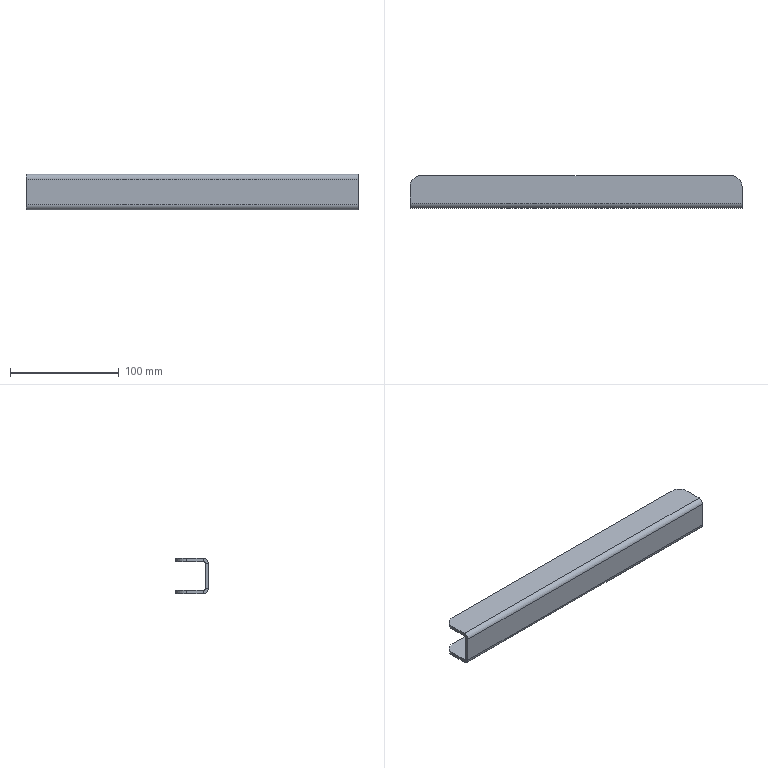Part | NX | features BREP 1 | 1 solid | 26 faces | box 304.8 x 29.997 x 32.461 mm | volume 76853 mm3 | plane 18 | cylinder 8 | commonest cylinder face diameters 19.964 x4 3.175 x2 9.22 x2
STEP:
#1=CARTESIAN_POINT('',(-152.4,0.,11.62));
#2=VERTEX_POINT('',#1);
#3=CARTESIAN_POINT('',(152.4,0.,11.62));
#4=VERTEX_POINT('',#3);
#5=CARTESIAN_POINT('',(-152.4,0.,11.62));
#6=DIRECTION('',(1.,0.,0.));
#7=VECTOR('',#6,1000.);
#8=LINE('',#5,#7);
#9=EDGE_CURVE('',#2,#4,#8,.T.);
#10=ORIENTED_EDGE('',*,*,#9,.T.);
#11=CARTESIAN_POINT('',(152.4,0.,-11.62));
#12=VERTEX_POINT('',#11);
#13=CARTESIAN_POINT('',(152.4,0.,11.62));
#14=DIRECTION('',(0.,0.,-1.));
#15=VECTOR('',#14,1000.);
#16=LINE('',#13,#15);
#17=EDGE_CURVE('',#4,#12,#16,.T.);
#18=ORIENTED_EDGE('',*,*,#17,.T.);
#19=CARTESIAN_POINT('',(-152.4,0.,-11.62));
#20=VERTEX_POINT('',#19);
#21=CARTESIAN_POINT('',(152.4,0.,-11.62));
#22=DIRECTION('',(-1.,0.,0.));
#23=VECTOR('',#22,1000.);
#24=LINE('',#21,#23);
#25=EDGE_CURVE('',#12,#20,#24,.T.);
#26=ORIENTED_EDGE('',*,*,#25,.T.);
#27=CARTESIAN_POINT('',(-152.4,0.,-11.62));
#28=DIRECTION('',(0.,0.,1.));
#29=VECTOR('',#28,1000.);
#30=LINE('',#27,#29);
#31=EDGE_CURVE('',#20,#2,#30,.T.);
#32=ORIENTED_EDGE('',*,*,#31,.T.);
#33=EDGE_LOOP('',(#10,#18,#26,#32));
#34=FACE_BOUND('',#33,.T.);
#35=CARTESIAN_POINT('',(0.,0.,0.));
#36=DIRECTION('',(0.,1.,0.));
#37=DIRECTION('',(1.,0.,0.));
#38=AXIS2_PLACEMENT_3D('',#35,#36,#37);
#39=PLANE('',#38);
#40=ADVANCED_FACE('',(#34),#39,.T.);
#41=CARTESIAN_POINT('',(-152.4,-3.023,-11.62));
#42=VERTEX_POINT('',#41);
#43=CARTESIAN_POINT('',(-152.4,0.,-11.62));
#44=DIRECTION('',(0.,-1.,0.));
#45=VECTOR('',#44,1000.);
#46=LINE('',#43,#45);
#47=EDGE_CURVE('',#20,#42,#46,.T.);
#48=ORIENTED_EDGE('',*,*,#47,.T.);
#49=CARTESIAN_POINT('',(-152.4,-3.023,11.62));
#50=VERTEX_POINT('',#49);
#51=CARTESIAN_POINT('',(-152.4,-3.023,-11.62));
#52=DIRECTION('',(0.,0.,1.));
#53=VECTOR('',#52,1000.);
#54=LINE('',#51,#53);
#55=EDGE_CURVE('',#42,#50,#54,.T.);
#56=ORIENTED_EDGE('',*,*,#55,.T.);
#57=CARTESIAN_POINT('',(-152.4,0.,11.62));
#58=DIRECTION('',(0.,-1.,0.));
#59=VECTOR('',#58,1000.);
#60=LINE('',#57,#59);
#61=EDGE_CURVE('',#2,#50,#60,.T.);
#62=ORIENTED_EDGE('',*,*,#61,.F.);
#63=ORIENTED_EDGE('',*,*,#31,.F.);
#64=EDGE_LOOP('',(#48,#56,#62,#63));
#65=FACE_BOUND('',#64,.T.);
#66=CARTESIAN_POINT('',(-152.4,-1.511,0.));
#67=DIRECTION('',(-1.,0.,0.));
#68=DIRECTION('',(0.,0.,1.));
#69=AXIS2_PLACEMENT_3D('',#66,#67,#68);
#70=PLANE('',#69);
#71=ADVANCED_FACE('',(#65),#70,.T.);
#72=ORIENTED_EDGE('',*,*,#61,.T.);
#73=CARTESIAN_POINT('',(-152.4,1.587,16.231));
#74=VERTEX_POINT('',#73);
#75=CARTESIAN_POINT('',(-152.4,1.587,11.62));
#76=DIRECTION('',(1.,0.,0.));
#77=DIRECTION('',(0.,0.,1.));
#78=AXIS2_PLACEMENT_3D('',#75,#76,#77);
#79=CIRCLE('',#78,4.61);
#80=EDGE_CURVE('',#74,#50,#79,.T.);
#81=ORIENTED_EDGE('',*,*,#80,.F.);
#82=CARTESIAN_POINT('',(-152.4,1.587,13.208));
#83=VERTEX_POINT('',#82);
#84=CARTESIAN_POINT('',(-152.4,1.587,13.208));
#85=DIRECTION('',(0.,0.,1.));
#86=VECTOR('',#85,1000.);
#87=LINE('',#84,#86);
#88=EDGE_CURVE('',#83,#74,#87,.T.);
#89=ORIENTED_EDGE('',*,*,#88,.F.);
#90=CARTESIAN_POINT('',(-152.4,1.587,11.62));
#91=DIRECTION('',(1.,0.,0.));
#92=DIRECTION('',(0.,0.,1.));
#93=AXIS2_PLACEMENT_3D('',#90,#91,#92);
#94=CIRCLE('',#93,1.587);
#95=EDGE_CURVE('',#83,#2,#94,.T.);
#96=ORIENTED_EDGE('',*,*,#95,.T.);
#97=EDGE_LOOP('',(#72,#81,#89,#96));
#98=FACE_BOUND('',#97,.T.);
#99=CARTESIAN_POINT('',(-152.4,-0.6037,13.812));
#100=DIRECTION('',(1.,0.,0.));
#101=DIRECTION('',(0.,1.,0.));
#102=AXIS2_PLACEMENT_3D('',#99,#100,#101);
#103=PLANE('',#102);
#104=ADVANCED_FACE('',(#98),#103,.F.);
#105=CARTESIAN_POINT('',(152.4,1.587,13.208));
#106=VERTEX_POINT('',#105);
#107=CARTESIAN_POINT('',(152.4,1.587,11.62));
#108=DIRECTION('',(1.,0.,0.));
#109=DIRECTION('',(0.,0.,1.));
#110=AXIS2_PLACEMENT_3D('',#107,#108,#109);
#111=CIRCLE('',#110,1.587);
#112=EDGE_CURVE('',#106,#4,#111,.T.);
#113=ORIENTED_EDGE('',*,*,#112,.T.);
#114=ORIENTED_EDGE('',*,*,#9,.F.);
#115=ORIENTED_EDGE('',*,*,#95,.F.);
#116=CARTESIAN_POINT('',(-152.4,1.587,13.208));
#117=DIRECTION('',(1.,0.,0.));
#118=VECTOR('',#117,1000.);
#119=LINE('',#116,#118);
#120=EDGE_CURVE('',#83,#106,#119,.T.);
#121=ORIENTED_EDGE('',*,*,#120,.T.);
#122=EDGE_LOOP('',(#113,#114,#115,#121));
#123=FACE_BOUND('',#122,.T.);
#124=CARTESIAN_POINT('',(-152.4,1.587,11.62));
#125=DIRECTION('',(1.,0.,0.));
#126=DIRECTION('',(0.,0.,1.));
#127=AXIS2_PLACEMENT_3D('',#124,#125,#126);
#128=CYLINDRICAL_SURFACE('',#127,1.587);
#129=ADVANCED_FACE('',(#123),#128,.F.);
#130=CARTESIAN_POINT('',(152.4,16.942,13.208));
#131=VERTEX_POINT('',#130);
#132=CARTESIAN_POINT('',(152.4,1.587,13.208));
#133=DIRECTION('',(0.,1.,0.));
#134=VECTOR('',#133,1000.);
#135=LINE('',#132,#134);
#136=EDGE_CURVE('',#106,#131,#135,.T.);
#137=ORIENTED_EDGE('',*,*,#136,.F.);
#138=ORIENTED_EDGE('',*,*,#120,.F.);
#139=CARTESIAN_POINT('',(-152.4,16.942,13.208));
#140=VERTEX_POINT('',#139);
#141=CARTESIAN_POINT('',(-152.4,16.942,13.208));
#142=DIRECTION('',(0.,-1.,0.));
#143=VECTOR('',#142,1000.);
#144=LINE('',#141,#143);
#145=EDGE_CURVE('',#140,#83,#144,.T.);
#146=ORIENTED_EDGE('',*,*,#145,.F.);
#147=CARTESIAN_POINT('',(-142.418,26.924,13.208));
#148=VERTEX_POINT('',#147);
#149=CARTESIAN_POINT('',(-142.418,16.942,13.208));
#150=DIRECTION('',(0.,0.,-1.));
#151=DIRECTION('',(-1.,0.,0.));
#152=AXIS2_PLACEMENT_3D('',#149,#150,#151);
#153=CIRCLE('',#152,9.982);
#154=EDGE_CURVE('',#140,#148,#153,.T.);
#155=ORIENTED_EDGE('',*,*,#154,.T.);
#156=CARTESIAN_POINT('',(142.418,26.924,13.208));
#157=VERTEX_POINT('',#156);
#158=CARTESIAN_POINT('',(142.418,26.924,13.208));
#159=DIRECTION('',(-1.,0.,0.));
#160=VECTOR('',#159,1000.);
#161=LINE('',#158,#160);
#162=EDGE_CURVE('',#157,#148,#161,.T.);
#163=ORIENTED_EDGE('',*,*,#162,.F.);
#164=CARTESIAN_POINT('',(142.418,16.942,13.208));
#165=DIRECTION('',(0.,0.,-1.));
#166=DIRECTION('',(0.,1.,0.));
#167=AXIS2_PLACEMENT_3D('',#164,#165,#166);
#168=CIRCLE('',#167,9.982);
#169=EDGE_CURVE('',#157,#131,#168,.T.);
#170=ORIENTED_EDGE('',*,*,#169,.T.);
#171=EDGE_LOOP('',(#137,#138,#146,#155,#163,#170));
#172=FACE_BOUND('',#171,.T.);
#173=CARTESIAN_POINT('',(-79.98,0.,13.208));
#174=DIRECTION('',(0.,0.,1.));
#175=DIRECTION('',(1.,0.,0.));
#176=AXIS2_PLACEMENT_3D('',#173,#174,#175);
#177=PLANE('',#176);
#178=ADVANCED_FACE('',(#172),#177,.F.);
#179=CARTESIAN_POINT('',(152.4,16.942,16.231));
#180=VERTEX_POINT('',#179);
#181=CARTESIAN_POINT('',(142.418,26.924,16.231));
#182=VERTEX_POINT('',#181);
#183=CARTESIAN_POINT('',(142.418,16.942,16.231));
#184=DIRECTION('',(0.,0.,1.));
#185=DIRECTION('',(1.,0.,0.));
#186=AXIS2_PLACEMENT_3D('',#183,#184,#185);
#187=CIRCLE('',#186,9.982);
#188=EDGE_CURVE('',#180,#182,#187,.T.);
#189=ORIENTED_EDGE('',*,*,#188,.F.);
#190=CARTESIAN_POINT('',(152.4,16.942,16.231));
#191=DIRECTION('',(0.,0.,-1.));
#192=VECTOR('',#191,1000.);
#193=LINE('',#190,#192);
#194=EDGE_CURVE('',#180,#131,#193,.T.);
#195=ORIENTED_EDGE('',*,*,#194,.T.);
#196=ORIENTED_EDGE('',*,*,#169,.F.);
#197=CARTESIAN_POINT('',(142.418,26.924,16.231));
#198=DIRECTION('',(0.,0.,-1.));
#199=VECTOR('',#198,1000.);
#200=LINE('',#197,#199);
#201=EDGE_CURVE('',#182,#157,#200,.T.);
#202=ORIENTED_EDGE('',*,*,#201,.F.);
#203=EDGE_LOOP('',(#189,#195,#196,#202));
#204=FACE_BOUND('',#203,.T.);
#205=CARTESIAN_POINT('',(142.418,16.942,16.681));
#206=DIRECTION('',(0.,0.,-1.));
#207=DIRECTION('',(0.,1.,0.));
#208=AXIS2_PLACEMENT_3D('',#205,#206,#207);
#209=CYLINDRICAL_SURFACE('',#208,9.982);
#210=ADVANCED_FACE('',(#204),#209,.T.);
#211=ORIENTED_EDGE('',*,*,#162,.T.);
#212=CARTESIAN_POINT('',(-142.418,26.924,16.231));
#213=VERTEX_POINT('',#212);
#214=CARTESIAN_POINT('',(-142.418,26.924,16.231));
#215=DIRECTION('',(0.,0.,-1.));
#216=VECTOR('',#215,1000.);
#217=LINE('',#214,#216);
#218=EDGE_CURVE('',#213,#148,#217,.T.);
#219=ORIENTED_EDGE('',*,*,#218,.F.);
#220=CARTESIAN_POINT('',(142.418,26.924,16.231));
#221=DIRECTION('',(-1.,0.,0.));
#222=VECTOR('',#221,1000.);
#223=LINE('',#220,#222);
#224=EDGE_CURVE('',#182,#213,#223,.T.);
#225=ORIENTED_EDGE('',*,*,#224,.F.);
#226=ORIENTED_EDGE('',*,*,#201,.T.);
#227=EDGE_LOOP('',(#211,#219,#225,#226));
#228=FACE_BOUND('',#227,.T.);
#229=CARTESIAN_POINT('',(0.,26.924,14.719));
#230=DIRECTION('',(0.,-1.,0.));
#231=DIRECTION('',(0.,0.,-1.));
#232=AXIS2_PLACEMENT_3D('',#229,#230,#231);
#233=PLANE('',#232);
#234=ADVANCED_FACE('',(#228),#233,.F.);
#235=ORIENTED_EDGE('',*,*,#224,.T.);
#236=CARTESIAN_POINT('',(-152.4,16.942,16.231));
#237=VERTEX_POINT('',#236);
#238=CARTESIAN_POINT('',(-142.418,16.942,16.231));
#239=DIRECTION('',(0.,0.,1.));
#240=DIRECTION('',(0.,1.,0.));
#241=AXIS2_PLACEMENT_3D('',#238,#239,#240);
#242=CIRCLE('',#241,9.982);
#243=EDGE_CURVE('',#213,#237,#242,.T.);
#244=ORIENTED_EDGE('',*,*,#243,.T.);
#245=CARTESIAN_POINT('',(-152.4,16.942,16.231));
#246=DIRECTION('',(0.,-1.,0.));
#247=VECTOR('',#246,1000.);
#248=LINE('',#245,#247);
#249=EDGE_CURVE('',#237,#74,#248,.T.);
#250=ORIENTED_EDGE('',*,*,#249,.T.);
#251=CARTESIAN_POINT('',(152.4,1.587,16.231));
#252=VERTEX_POINT('',#251);
#253=CARTESIAN_POINT('',(-152.4,1.587,16.231));
#254=DIRECTION('',(1.,0.,0.));
#255=VECTOR('',#254,1000.);
#256=LINE('',#253,#255);
#257=EDGE_CURVE('',#74,#252,#256,.T.);
#258=ORIENTED_EDGE('',*,*,#257,.T.);
#259=CARTESIAN_POINT('',(152.4,1.587,16.231));
#260=DIRECTION('',(0.,1.,0.));
#261=VECTOR('',#260,1000.);
#262=LINE('',#259,#261);
#263=EDGE_CURVE('',#252,#180,#262,.T.);
#264=ORIENTED_EDGE('',*,*,#263,.T.);
#265=ORIENTED_EDGE('',*,*,#188,.T.);
#266=EDGE_LOOP('',(#235,#244,#250,#258,#264,#265));
#267=FACE_BOUND('',#266,.T.);
#268=CARTESIAN_POINT('',(-79.98,0.,16.231));
#269=DIRECTION('',(0.,0.,1.));
#270=DIRECTION('',(1.,0.,0.));
#271=AXIS2_PLACEMENT_3D('',#268,#269,#270);
#272=PLANE('',#271);
#273=ADVANCED_FACE('',(#267),#272,.T.);
#274=ORIENTED_EDGE('',*,*,#263,.F.);
#275=CARTESIAN_POINT('',(152.4,1.587,13.208));
#276=DIRECTION('',(0.,0.,1.));
#277=VECTOR('',#276,1000.);
#278=LINE('',#275,#277);
#279=EDGE_CURVE('',#106,#252,#278,.T.);
#280=ORIENTED_EDGE('',*,*,#279,.F.);
#281=ORIENTED_EDGE('',*,*,#136,.T.);
#282=ORIENTED_EDGE('',*,*,#194,.F.);
#283=EDGE_LOOP('',(#274,#280,#281,#282));
#284=FACE_BOUND('',#283,.T.);
#285=CARTESIAN_POINT('',(152.4,14.256,14.719));
#286=DIRECTION('',(-1.,0.,0.));
#287=DIRECTION('',(0.,0.,1.));
#288=AXIS2_PLACEMENT_3D('',#285,#286,#287);
#289=PLANE('',#288);
#290=ADVANCED_FACE('',(#284),#289,.F.);
#291=ORIENTED_EDGE('',*,*,#279,.T.);
#292=CARTESIAN_POINT('',(152.4,-3.023,11.62));
#293=VERTEX_POINT('',#292);
#294=CARTESIAN_POINT('',(152.4,1.587,11.62));
#295=DIRECTION('',(1.,0.,0.));
#296=DIRECTION('',(0.,0.,1.));
#297=AXIS2_PLACEMENT_3D('',#294,#295,#296);
#298=CIRCLE('',#297,4.61);
#299=EDGE_CURVE('',#252,#293,#298,.T.);
#300=ORIENTED_EDGE('',*,*,#299,.T.);
#301=CARTESIAN_POINT('',(152.4,0.,11.62));
#302=DIRECTION('',(0.,-1.,0.));
#303=VECTOR('',#302,1000.);
#304=LINE('',#301,#303);
#305=EDGE_CURVE('',#4,#293,#304,.T.);
#306=ORIENTED_EDGE('',*,*,#305,.F.);
#307=ORIENTED_EDGE('',*,*,#112,.F.);
#308=EDGE_LOOP('',(#291,#300,#306,#307));
#309=FACE_BOUND('',#308,.T.);
#310=CARTESIAN_POINT('',(152.4,-0.6037,13.812));
#311=DIRECTION('',(1.,0.,0.));
#312=DIRECTION('',(0.,1.,0.));
#313=AXIS2_PLACEMENT_3D('',#310,#311,#312);
#314=PLANE('',#313);
#315=ADVANCED_FACE('',(#309),#314,.T.);
#316=ORIENTED_EDGE('',*,*,#305,.T.);
#317=CARTESIAN_POINT('',(152.4,-3.023,-11.62));
#318=VERTEX_POINT('',#317);
#319=CARTESIAN_POINT('',(152.4,-3.023,11.62));
#320=DIRECTION('',(0.,0.,-1.));
#321=VECTOR('',#320,1000.);
#322=LINE('',#319,#321);
#323=EDGE_CURVE('',#293,#318,#322,.T.);
#324=ORIENTED_EDGE('',*,*,#323,.T.);
#325=CARTESIAN_POINT('',(152.4,0.,-11.62));
#326=DIRECTION('',(0.,-1.,0.));
#327=VECTOR('',#326,1000.);
#328=LINE('',#325,#327);
#329=EDGE_CURVE('',#12,#318,#328,.T.);
#330=ORIENTED_EDGE('',*,*,#329,.F.);
#331=ORIENTED_EDGE('',*,*,#17,.F.);
#332=EDGE_LOOP('',(#316,#324,#330,#331));
#333=FACE_BOUND('',#332,.T.);
#334=CARTESIAN_POINT('',(152.4,-1.511,0.));
#335=DIRECTION('',(1.,0.,0.));
#336=DIRECTION('',(0.,1.,0.));
#337=AXIS2_PLACEMENT_3D('',#334,#335,#336);
#338=PLANE('',#337);
#339=ADVANCED_FACE('',(#333),#338,.T.);
#340=ORIENTED_EDGE('',*,*,#329,.T.);
#341=CARTESIAN_POINT('',(152.4,1.587,-16.231));
#342=VERTEX_POINT('',#341);
#343=CARTESIAN_POINT('',(152.4,1.587,-11.62));
#344=DIRECTION('',(-1.,0.,0.));
#345=DIRECTION('',(0.,0.,-1.));
#346=AXIS2_PLACEMENT_3D('',#343,#344,#345);
#347=CIRCLE('',#346,4.61);
#348=EDGE_CURVE('',#342,#318,#347,.T.);
#349=ORIENTED_EDGE('',*,*,#348,.F.);
#350=CARTESIAN_POINT('',(152.4,1.587,-13.208));
#351=VERTEX_POINT('',#350);
#352=CARTESIAN_POINT('',(152.4,1.587,-13.208));
#353=DIRECTION('',(0.,0.,-1.));
#354=VECTOR('',#353,1000.);
#355=LINE('',#352,#354);
#356=EDGE_CURVE('',#351,#342,#355,.T.);
#357=ORIENTED_EDGE('',*,*,#356,.F.);
#358=CARTESIAN_POINT('',(152.4,1.587,-11.62));
#359=DIRECTION('',(-1.,0.,0.));
#360=DIRECTION('',(0.,0.,-1.));
#361=AXIS2_PLACEMENT_3D('',#358,#359,#360);
#362=CIRCLE('',#361,1.587);
#363=EDGE_CURVE('',#351,#12,#362,.T.);
#364=ORIENTED_EDGE('',*,*,#363,.T.);
#365=EDGE_LOOP('',(#340,#349,#357,#364));
#366=FACE_BOUND('',#365,.T.);
#367=CARTESIAN_POINT('',(152.4,-0.6037,-13.812));
#368=DIRECTION('',(-1.,0.,0.));
#369=DIRECTION('',(0.,0.,1.));
#370=AXIS2_PLACEMENT_3D('',#367,#368,#369);
#371=PLANE('',#370);
#372=ADVANCED_FACE('',(#366),#371,.F.);
#373=CARTESIAN_POINT('',(-152.4,1.587,-13.208));
#374=VERTEX_POINT('',#373);
#375=CARTESIAN_POINT('',(-152.4,1.587,-11.62));
#376=DIRECTION('',(-1.,0.,0.));
#377=DIRECTION('',(0.,0.,-1.));
#378=AXIS2_PLACEMENT_3D('',#375,#376,#377);
#379=CIRCLE('',#378,1.587);
#380=EDGE_CURVE('',#374,#20,#379,.T.);
#381=ORIENTED_EDGE('',*,*,#380,.T.);
#382=ORIENTED_EDGE('',*,*,#25,.F.);
#383=ORIENTED_EDGE('',*,*,#363,.F.);
#384=CARTESIAN_POINT('',(152.4,1.587,-13.208));
#385=DIRECTION('',(-1.,0.,0.));
#386=VECTOR('',#385,1000.);
#387=LINE('',#384,#386);
#388=EDGE_CURVE('',#351,#374,#387,.T.);
#389=ORIENTED_EDGE('',*,*,#388,.T.);
#390=EDGE_LOOP('',(#381,#382,#383,#389));
#391=FACE_BOUND('',#390,.T.);
#392=CARTESIAN_POINT('',(152.4,1.587,-11.62));
#393=DIRECTION('',(-1.,0.,0.));
#394=DIRECTION('',(0.,0.,-1.));
#395=AXIS2_PLACEMENT_3D('',#392,#393,#394);
#396=CYLINDRICAL_SURFACE('',#395,1.587);
#397=ADVANCED_FACE('',(#391),#396,.F.);
#398=CARTESIAN_POINT('',(-142.418,26.975,-13.208));
#399=VERTEX_POINT('',#398);
#400=CARTESIAN_POINT('',(142.418,26.975,-13.208));
#401=VERTEX_POINT('',#400);
#402=CARTESIAN_POINT('',(-142.418,26.975,-13.208));
#403=DIRECTION('',(1.,0.,0.));
#404=VECTOR('',#403,1000.);
#405=LINE('',#402,#404);
#406=EDGE_CURVE('',#399,#401,#405,.T.);
#407=ORIENTED_EDGE('',*,*,#406,.F.);
#408=CARTESIAN_POINT('',(-152.4,16.993,-13.208));
#409=VERTEX_POINT('',#408);
#410=CARTESIAN_POINT('',(-142.418,16.993,-13.208));
#411=DIRECTION('',(0.,0.,1.));
#412=DIRECTION('',(0.,1.,0.));
#413=AXIS2_PLACEMENT_3D('',#410,#411,#412);
#414=CIRCLE('',#413,9.982);
#415=EDGE_CURVE('',#399,#409,#414,.T.);
#416=ORIENTED_EDGE('',*,*,#415,.T.);
#417=CARTESIAN_POINT('',(-152.4,1.587,-13.208));
#418=DIRECTION('',(0.,1.,0.));
#419=VECTOR('',#418,1000.);
#420=LINE('',#417,#419);
#421=EDGE_CURVE('',#374,#409,#420,.T.);
#422=ORIENTED_EDGE('',*,*,#421,.F.);
#423=ORIENTED_EDGE('',*,*,#388,.F.);
#424=CARTESIAN_POINT('',(152.4,16.993,-13.208));
#425=VERTEX_POINT('',#424);
#426=CARTESIAN_POINT('',(152.4,16.993,-13.208));
#427=DIRECTION('',(0.,-1.,0.));
#428=VECTOR('',#427,1000.);
#429=LINE('',#426,#428);
#430=EDGE_CURVE('',#425,#351,#429,.T.);
#431=ORIENTED_EDGE('',*,*,#430,.F.);
#432=CARTESIAN_POINT('',(142.418,16.993,-13.208));
#433=DIRECTION('',(0.,0.,1.));
#434=DIRECTION('',(1.,0.,0.));
#435=AXIS2_PLACEMENT_3D('',#432,#433,#434);
#436=CIRCLE('',#435,9.982);
#437=EDGE_CURVE('',#425,#401,#436,.T.);
#438=ORIENTED_EDGE('',*,*,#437,.T.);
#439=EDGE_LOOP('',(#407,#416,#422,#423,#431,#438));
#440=FACE_BOUND('',#439,.T.);
#441=CARTESIAN_POINT('',(79.98,0.,-13.208));
#442=DIRECTION('',(0.,0.,-1.));
#443=DIRECTION('',(0.,-1.,0.));
#444=AXIS2_PLACEMENT_3D('',#441,#442,#443);
#445=PLANE('',#444);
#446=ADVANCED_FACE('',(#440),#445,.F.);
#447=CARTESIAN_POINT('',(142.418,26.975,-16.231));
#448=VERTEX_POINT('',#447);
#449=CARTESIAN_POINT('',(152.4,16.993,-16.231));
#450=VERTEX_POINT('',#449);
#451=CARTESIAN_POINT('',(142.418,16.993,-16.231));
#452=DIRECTION('',(0.,0.,-1.));
#453=DIRECTION('',(0.,1.,0.));
#454=AXIS2_PLACEMENT_3D('',#451,#452,#453);
#455=CIRCLE('',#454,9.982);
#456=EDGE_CURVE('',#448,#450,#455,.T.);
#457=ORIENTED_EDGE('',*,*,#456,.F.);
#458=CARTESIAN_POINT('',(142.418,26.975,-16.231));
#459=DIRECTION('',(0.,0.,1.));
#460=VECTOR('',#459,1000.);
#461=LINE('',#458,#460);
#462=EDGE_CURVE('',#448,#401,#461,.T.);
#463=ORIENTED_EDGE('',*,*,#462,.T.);
#464=ORIENTED_EDGE('',*,*,#437,.F.);
#465=CARTESIAN_POINT('',(152.4,16.993,-16.231));
#466=DIRECTION('',(0.,0.,1.));
#467=VECTOR('',#466,1000.);
#468=LINE('',#465,#467);
#469=EDGE_CURVE('',#450,#425,#468,.T.);
#470=ORIENTED_EDGE('',*,*,#469,.F.);
#471=EDGE_LOOP('',(#457,#463,#464,#470));
#472=FACE_BOUND('',#471,.T.);
#473=CARTESIAN_POINT('',(142.418,16.993,-16.681));
#474=DIRECTION('',(0.,0.,1.));
#475=DIRECTION('',(1.,0.,0.));
#476=AXIS2_PLACEMENT_3D('',#473,#474,#475);
#477=CYLINDRICAL_SURFACE('',#476,9.982);
#478=ADVANCED_FACE('',(#472),#477,.T.);
#479=ORIENTED_EDGE('',*,*,#430,.T.);
#480=ORIENTED_EDGE('',*,*,#356,.T.);
#481=CARTESIAN_POINT('',(152.4,16.993,-16.231));
#482=DIRECTION('',(0.,-1.,0.));
#483=VECTOR('',#482,1000.);
#484=LINE('',#481,#483);
#485=EDGE_CURVE('',#450,#342,#484,.T.);
#486=ORIENTED_EDGE('',*,*,#485,.F.);
#487=ORIENTED_EDGE('',*,*,#469,.T.);
#488=EDGE_LOOP('',(#479,#480,#486,#487));
#489=FACE_BOUND('',#488,.T.);
#490=CARTESIAN_POINT('',(152.4,14.281,-14.719));
#491=DIRECTION('',(-1.,0.,0.));
#492=DIRECTION('',(0.,0.,1.));
#493=AXIS2_PLACEMENT_3D('',#490,#491,#492);
#494=PLANE('',#493);
#495=ADVANCED_FACE('',(#489),#494,.F.);
#496=ORIENTED_EDGE('',*,*,#485,.T.);
#497=CARTESIAN_POINT('',(-152.4,1.587,-16.231));
#498=VERTEX_POINT('',#497);
#499=CARTESIAN_POINT('',(152.4,1.587,-16.231));
#500=DIRECTION('',(-1.,0.,0.));
#501=VECTOR('',#500,1000.);
#502=LINE('',#499,#501);
#503=EDGE_CURVE('',#342,#498,#502,.T.);
#504=ORIENTED_EDGE('',*,*,#503,.T.);
#505=CARTESIAN_POINT('',(-152.4,16.993,-16.231));
#506=VERTEX_POINT('',#505);
#507=CARTESIAN_POINT('',(-152.4,1.587,-16.231));
#508=DIRECTION('',(0.,1.,0.));
#509=VECTOR('',#508,1000.);
#510=LINE('',#507,#509);
#511=EDGE_CURVE('',#498,#506,#510,.T.);
#512=ORIENTED_EDGE('',*,*,#511,.T.);
#513=CARTESIAN_POINT('',(-142.418,26.975,-16.231));
#514=VERTEX_POINT('',#513);
#515=CARTESIAN_POINT('',(-142.418,16.993,-16.231));
#516=DIRECTION('',(0.,0.,-1.));
#517=DIRECTION('',(-1.,0.,0.));
#518=AXIS2_PLACEMENT_3D('',#515,#516,#517);
#519=CIRCLE('',#518,9.982);
#520=EDGE_CURVE('',#506,#514,#519,.T.);
#521=ORIENTED_EDGE('',*,*,#520,.T.);
#522=CARTESIAN_POINT('',(-142.418,26.975,-16.231));
#523=DIRECTION('',(1.,0.,0.));
#524=VECTOR('',#523,1000.);
#525=LINE('',#522,#524);
#526=EDGE_CURVE('',#514,#448,#525,.T.);
#527=ORIENTED_EDGE('',*,*,#526,.T.);
#528=ORIENTED_EDGE('',*,*,#456,.T.);
#529=EDGE_LOOP('',(#496,#504,#512,#521,#527,#528));
#530=FACE_BOUND('',#529,.T.);
#531=CARTESIAN_POINT('',(79.98,0.,-16.231));
#532=DIRECTION('',(0.,0.,-1.));
#533=DIRECTION('',(0.,-1.,0.));
#534=AXIS2_PLACEMENT_3D('',#531,#532,#533);
#535=PLANE('',#534);
#536=ADVANCED_FACE('',(#530),#535,.T.);
#537=ORIENTED_EDGE('',*,*,#526,.F.);
#538=CARTESIAN_POINT('',(-142.418,26.975,-16.231));
#539=DIRECTION('',(0.,0.,1.));
#540=VECTOR('',#539,1000.);
#541=LINE('',#538,#540);
#542=EDGE_CURVE('',#514,#399,#541,.T.);
#543=ORIENTED_EDGE('',*,*,#542,.T.);
#544=ORIENTED_EDGE('',*,*,#406,.T.);
#545=ORIENTED_EDGE('',*,*,#462,.F.);
#546=EDGE_LOOP('',(#537,#543,#544,#545));
#547=FACE_BOUND('',#546,.T.);
#548=CARTESIAN_POINT('',(0.,26.975,-14.719));
#549=DIRECTION('',(0.,-1.,0.));
#550=DIRECTION('',(0.,0.,-1.));
#551=AXIS2_PLACEMENT_3D('',#548,#549,#550);
#552=PLANE('',#551);
#553=ADVANCED_FACE('',(#547),#552,.F.);
#554=ORIENTED_EDGE('',*,*,#520,.F.);
#555=CARTESIAN_POINT('',(-152.4,16.993,-16.231));
#556=DIRECTION('',(0.,0.,1.));
#557=VECTOR('',#556,1000.);
#558=LINE('',#555,#557);
#559=EDGE_CURVE('',#506,#409,#558,.T.);
#560=ORIENTED_EDGE('',*,*,#559,.T.);
#561=ORIENTED_EDGE('',*,*,#415,.F.);
#562=ORIENTED_EDGE('',*,*,#542,.F.);
#563=EDGE_LOOP('',(#554,#560,#561,#562));
#564=FACE_BOUND('',#563,.T.);
#565=CARTESIAN_POINT('',(-142.418,16.993,-16.681));
#566=DIRECTION('',(0.,0.,1.));
#567=DIRECTION('',(0.,1.,0.));
#568=AXIS2_PLACEMENT_3D('',#565,#566,#567);
#569=CYLINDRICAL_SURFACE('',#568,9.982);
#570=ADVANCED_FACE('',(#564),#569,.T.);
#571=ORIENTED_EDGE('',*,*,#511,.F.);
#572=CARTESIAN_POINT('',(-152.4,1.587,-13.208));
#573=DIRECTION('',(0.,0.,-1.));
#574=VECTOR('',#573,1000.);
#575=LINE('',#572,#574);
#576=EDGE_CURVE('',#374,#498,#575,.T.);
#577=ORIENTED_EDGE('',*,*,#576,.F.);
#578=ORIENTED_EDGE('',*,*,#421,.T.);
#579=ORIENTED_EDGE('',*,*,#559,.F.);
#580=EDGE_LOOP('',(#571,#577,#578,#579));
#581=FACE_BOUND('',#580,.T.);
#582=CARTESIAN_POINT('',(-152.4,14.281,-14.719));
#583=DIRECTION('',(1.,0.,0.));
#584=DIRECTION('',(0.,1.,0.));
#585=AXIS2_PLACEMENT_3D('',#582,#583,#584);
#586=PLANE('',#585);
#587=ADVANCED_FACE('',(#581),#586,.F.);
#588=ORIENTED_EDGE('',*,*,#576,.T.);
#589=CARTESIAN_POINT('',(-152.4,1.587,-11.62));
#590=DIRECTION('',(-1.,0.,0.));
#591=DIRECTION('',(0.,0.,-1.));
#592=AXIS2_PLACEMENT_3D('',#589,#590,#591);
#593=CIRCLE('',#592,4.61);
#594=EDGE_CURVE('',#498,#42,#593,.T.);
#595=ORIENTED_EDGE('',*,*,#594,.T.);
#596=ORIENTED_EDGE('',*,*,#47,.F.);
#597=ORIENTED_EDGE('',*,*,#380,.F.);
#598=EDGE_LOOP('',(#588,#595,#596,#597));
#599=FACE_BOUND('',#598,.T.);
#600=CARTESIAN_POINT('',(-152.4,-0.6037,-13.812));
#601=DIRECTION('',(-1.,0.,0.));
#602=DIRECTION('',(0.,0.,1.));
#603=AXIS2_PLACEMENT_3D('',#600,#601,#602);
#604=PLANE('',#603);
#605=ADVANCED_FACE('',(#599),#604,.T.);
#606=ORIENTED_EDGE('',*,*,#348,.T.);
#607=CARTESIAN_POINT('',(152.4,-3.023,-11.62));
#608=DIRECTION('',(-1.,0.,0.));
#609=VECTOR('',#608,1000.);
#610=LINE('',#607,#609);
#611=EDGE_CURVE('',#318,#42,#610,.T.);
#612=ORIENTED_EDGE('',*,*,#611,.T.);
#613=ORIENTED_EDGE('',*,*,#594,.F.);
#614=ORIENTED_EDGE('',*,*,#503,.F.);
#615=EDGE_LOOP('',(#606,#612,#613,#614));
#616=FACE_BOUND('',#615,.T.);
#617=CARTESIAN_POINT('',(152.4,1.587,-11.62));
#618=DIRECTION('',(-1.,0.,0.));
#619=DIRECTION('',(0.,0.,-1.));
#620=AXIS2_PLACEMENT_3D('',#617,#618,#619);
#621=CYLINDRICAL_SURFACE('',#620,4.61);
#622=ADVANCED_FACE('',(#616),#621,.T.);
#623=ORIENTED_EDGE('',*,*,#611,.F.);
#624=ORIENTED_EDGE('',*,*,#323,.F.);
#625=CARTESIAN_POINT('',(-152.4,-3.023,11.62));
#626=DIRECTION('',(1.,0.,0.));
#627=VECTOR('',#626,1000.);
#628=LINE('',#625,#627);
#629=EDGE_CURVE('',#50,#293,#628,.T.);
#630=ORIENTED_EDGE('',*,*,#629,.F.);
#631=ORIENTED_EDGE('',*,*,#55,.F.);
#632=EDGE_LOOP('',(#623,#624,#630,#631));
#633=FACE_BOUND('',#632,.T.);
#634=CARTESIAN_POINT('',(0.,-3.023,0.));
#635=DIRECTION('',(0.,1.,0.));
#636=DIRECTION('',(1.,0.,0.));
#637=AXIS2_PLACEMENT_3D('',#634,#635,#636);
#638=PLANE('',#637);
#639=ADVANCED_FACE('',(#633),#638,.F.);
#640=ORIENTED_EDGE('',*,*,#80,.T.);
#641=ORIENTED_EDGE('',*,*,#629,.T.);
#642=ORIENTED_EDGE('',*,*,#299,.F.);
#643=ORIENTED_EDGE('',*,*,#257,.F.);
#644=EDGE_LOOP('',(#640,#641,#642,#643));
#645=FACE_BOUND('',#644,.T.);
#646=CARTESIAN_POINT('',(-152.4,1.587,11.62));
#647=DIRECTION('',(1.,0.,0.));
#648=DIRECTION('',(0.,0.,1.));
#649=AXIS2_PLACEMENT_3D('',#646,#647,#648);
#650=CYLINDRICAL_SURFACE('',#649,4.61);
#651=ADVANCED_FACE('',(#645),#650,.T.);
#652=ORIENTED_EDGE('',*,*,#145,.T.);
#653=ORIENTED_EDGE('',*,*,#88,.T.);
#654=ORIENTED_EDGE('',*,*,#249,.F.);
#655=CARTESIAN_POINT('',(-152.4,16.942,16.231));
#656=DIRECTION('',(0.,0.,-1.));
#657=VECTOR('',#656,1000.);
#658=LINE('',#655,#657);
#659=EDGE_CURVE('',#237,#140,#658,.T.);
#660=ORIENTED_EDGE('',*,*,#659,.T.);
#661=EDGE_LOOP('',(#652,#653,#654,#660));
#662=FACE_BOUND('',#661,.T.);
#663=CARTESIAN_POINT('',(-152.4,14.256,14.719));
#664=DIRECTION('',(1.,0.,0.));
#665=DIRECTION('',(0.,1.,0.));
#666=AXIS2_PLACEMENT_3D('',#663,#664,#665);
#667=PLANE('',#666);
#668=ADVANCED_FACE('',(#662),#667,.F.);
#669=ORIENTED_EDGE('',*,*,#243,.F.);
#670=ORIENTED_EDGE('',*,*,#218,.T.);
#671=ORIENTED_EDGE('',*,*,#154,.F.);
#672=ORIENTED_EDGE('',*,*,#659,.F.);
#673=EDGE_LOOP('',(#669,#670,#671,#672));
#674=FACE_BOUND('',#673,.T.);
#675=CARTESIAN_POINT('',(-142.418,16.942,16.681));
#676=DIRECTION('',(0.,0.,-1.));
#677=DIRECTION('',(-1.,0.,0.));
#678=AXIS2_PLACEMENT_3D('',#675,#676,#677);
#679=CYLINDRICAL_SURFACE('',#678,9.982);
#680=ADVANCED_FACE('',(#674),#679,.T.);
#681=CLOSED_SHELL('',(#40,#71,#104,#129,#178,#210,#234,#273,#290,#315,#339,#372,#397,#446,#478,#495,#536,#553,#570,#587,#605,#622,#639,#651,#668,#680));
#682=MANIFOLD_SOLID_BREP('',#681);
#683=(LENGTH_UNIT()NAMED_UNIT(*)SI_UNIT(.MILLI.,.METRE.));
#684=UNCERTAINTY_MEASURE_WITH_UNIT(LENGTH_MEASURE(0.00001),#683,'','');
#685=(NAMED_UNIT(*)PLANE_ANGLE_UNIT()SI_UNIT($,.RADIAN.));
#686=(NAMED_UNIT(*)SI_UNIT($,.STERADIAN.)SOLID_ANGLE_UNIT());
#687=(GEOMETRIC_REPRESENTATION_CONTEXT(3)GLOBAL_UNCERTAINTY_ASSIGNED_CONTEXT((#684))GLOBAL_UNIT_ASSIGNED_CONTEXT((#683,#685,#686))REPRESENTATION_CONTEXT('',''));
#688=ADVANCED_BREP_SHAPE_REPRESENTATION('',(#682),#687);